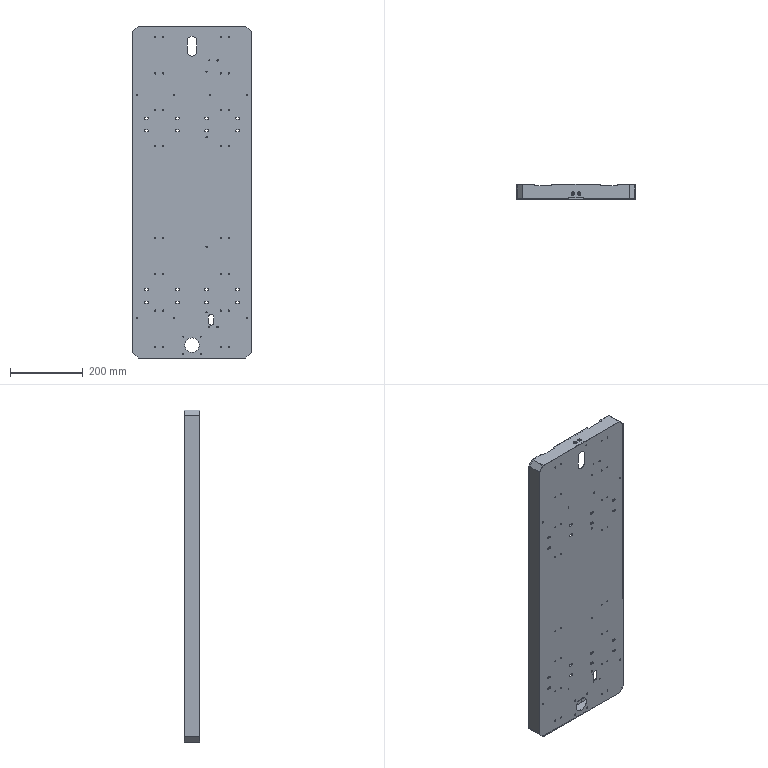Part | SolidWorks | features BaseBody 1 | 1 solid | 319 faces | box 325 x 42 x 910 mm | volume 886307 mm3 | cylinder 211 | plane 108 | commonest cylinder face diameters 3.3 x110 6 x32 7.9 x28 2.5 x20 4.2 x4 5 x4